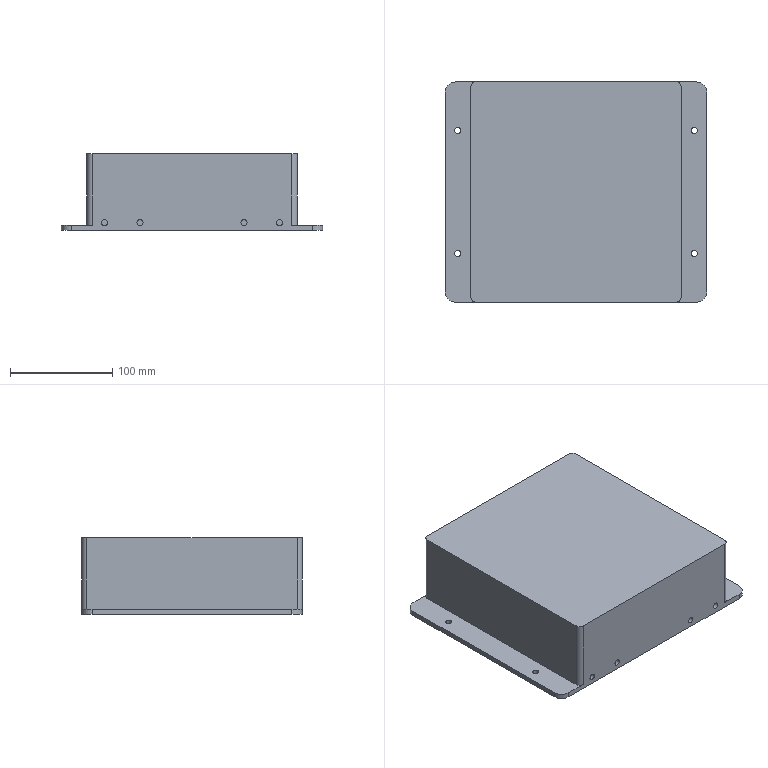NC program | NX | posted with a generic post | part box 255 x 215 x 75 mm
Lines 12222 to 12583 of 12583:
(ZLEVEL_PROFILE_COPY_1_COPY , TOOL : D10JING)
N24430 T14 M6
N24432 G54
N24434 G17 G0 G90 X-1.732 Y114.5 B0. C0. S9500 M3
N24436 G43 Z30. H14
N24438 Z-12.
N24440 G94 G1 Z-15. F1000.
N24442 X-0.866 Y113.
N24444 G3 X0. Y112.5 R1.
N24446 G1 X117.5 F1200.
N24448 G2 X132.5 Y97.5 R15.
N24450 G1 Y-97.5
N24452 G2 X117.5 Y-112.5 R15.
N24454 G1 X-117.5
N24456 G2 X-132.5 Y-97.5 R15.
N24458 G1 Y97.5
N24460 G2 X-117.5 Y112.5 R15.
N24462 G1 X0.
N24464 G3 X0.866 Y113. R1.
N24466 G1 X1.732 Y114.5
N24468 Z-14.
N24470 G0 Z30.
N24472 X-1.732
N24474 Z-27.
N24476 G1 Z-30. F1000.
N24478 X-0.866 Y113.
N24480 G3 X0. Y112.5 R1.
N24482 G1 X117.5 F1200.
N24484 G2 X132.5 Y97.5 R15.
N24486 G1 Y-97.5
N24488 G2 X117.5 Y-112.5 R15.
N24490 G1 X-117.5
N24492 G2 X-132.5 Y-97.5 R15.
N24494 G1 Y97.5
N24496 G2 X-117.5 Y112.5 R15.
N24498 G1 X0.
N24500 G3 X0.866 Y113. R1.
N24502 G1 X1.732 Y114.5
N24504 Z-29.
N24506 G0 Z30.
N24508 X-1.732
N24510 Z-42.
N24512 G1 Z-45. F1000.
N24514 X-0.866 Y113.
N24516 G3 X0. Y112.5 R1.
N24518 G1 X117.5 F1200.
N24520 G2 X132.5 Y97.5 R15.
N24522 G1 Y-97.5
N24524 G2 X117.5 Y-112.5 R15.
N24526 G1 X-117.5
N24528 G2 X-132.5 Y-97.5 R15.
N24530 G1 Y97.5
N24532 G2 X-117.5 Y112.5 R15.
N24534 G1 X0.
N24536 G3 X0.866 Y113. R1.
N24538 G1 X1.732 Y114.5
N24540 Z-44.
N24542 G0 Z30.
N24544 X-1.732
N24546 Z-57.
N24548 G1 Z-60. F1000.
N24550 X-0.866 Y113.
N24552 G3 X0. Y112.5 R1.
N24554 G1 X117.5 F1200.
N24556 G2 X132.5 Y97.5 R15.
N24558 G1 Y-97.5
N24560 G2 X117.5 Y-112.5 R15.
N24562 G1 X-117.5
N24564 G2 X-132.5 Y-97.5 R15.
N24566 G1 Y97.5
N24568 G2 X-117.5 Y112.5 R15.
N24570 G1 X0.
N24572 G3 X0.866 Y113. R1.
N24574 G1 X1.732 Y114.5
N24576 Z-59.
N24578 G0 Z30.
N24580 X-1.732
N24582 Z-72.
N24584 G1 Z-75. F1000.
N24586 X-0.866 Y113.
N24588 G3 X0. Y112.5 R1.
N24590 G1 X117.5 F1200.
N24592 G2 X132.5 Y97.5 R15.
N24594 G1 Y-97.5
N24596 G2 X117.5 Y-112.5 R15.
N24598 G1 X-117.5
N24600 G2 X-132.5 Y-97.5 R15.
N24602 G1 Y97.5
N24604 G2 X-117.5 Y112.5 R15.
N24606 G1 X0.
N24608 G3 X0.866 Y113. R1.
N24610 G1 X1.732 Y114.5
N24612 Z-74.
N24614 G0 Z30.
(ZLEVEL_PROFILE_COPY_1_COPY_COPY , TOOL : D10JING)
N24616 X95.656
N24618 Z-10.98
N24620 G1 Z-13.98 F1000.
N24622 X96.496 Y113.009
N24624 G3 X97.357 Y112.5 R1.
N24626 G1 X97.797 Y112.495 F1200.
N24628 X97.854 Y112.494
N24630 G2 X107.5 Y102.5 R10.
N24632 G1 Y-102.5
N24634 G2 X97.86 Y-112.494 R10.
N24636 G1 X97.797 Y-112.495
N24638 X97.357 Y-112.5
N24640 G3 X96.496 Y-113.009 R1.
N24642 G1 X95.656 Y-114.5
N24644 Z-12.98
N24646 G0 Z30.
N24648 X95.654 Y114.5
N24650 Z-24.96
N24652 G1 Z-27.96 F1000.
N24654 X96.496 Y113.009
N24656 G3 X97.357 Y112.5 R1.
N24658 G1 X97.797 Y112.496 F1200.
N24660 X97.854 Y112.494
N24662 G2 X107.5 Y102.5 R10.
N24664 G1 Y-102.5
N24666 G2 X97.86 Y-112.494 R10.
N24668 G1 X97.797 Y-112.496
N24670 X97.357 Y-112.5
N24672 G3 X96.496 Y-113.009 R1.
N24674 G1 X95.654 Y-114.5
N24676 Z-26.96
N24678 G0 Z30.
N24680 X95.653 Y114.5
N24682 Z-38.94
N24684 G1 Z-41.94 F1000.
N24686 X96.495 Y113.008
N24688 G3 X97.357 Y112.5 R1.
N24690 G1 X97.797 Y112.496 F1200.
N24692 X97.854 Y112.494
N24694 G2 X107.5 Y102.5 R10.
N24696 G1 Y-102.5
N24698 G2 X97.797 Y-112.496 R10.
N24700 G1 X97.357 Y-112.5
N24702 G3 X96.495 Y-113.008 R1.
N24704 G1 X95.653 Y-114.5
N24706 Z-40.94
N24708 G0 Z30.
N24710 X95.651 Y114.5
N24712 Z-52.92
N24714 G1 Z-55.92 F1000.
N24716 X96.495 Y113.008
N24718 G3 X97.357 Y112.5 R1.
N24720 G1 X97.797 Y112.496 F1200.
N24722 X97.83 Y112.495
N24724 G2 X107.5 Y102.5 R10.
N24726 G1 Y-102.5
N24728 G2 X97.797 Y-112.496 R10.001
N24730 G1 X97.357 Y-112.5
N24732 G3 X96.495 Y-113.008 R1.
N24734 G1 X95.651 Y-114.5
N24736 Z-54.92
N24738 G0 Z30.
N24740 X95.649 Y114.5
N24742 Z-66.9
N24744 G1 Z-69.9 F1000.
N24746 X96.495 Y113.007
N24748 G3 X97.357 Y112.5 R1.
N24750 G1 X97.797 Y112.496 F1200.
N24752 X97.83 Y112.495
N24754 G2 X107.5 Y102.5 R10.
N24756 G1 Y-102.5
N24758 G2 X97.797 Y-112.496 R10.001
N24760 G1 X97.357 Y-112.5
N24762 G3 X96.495 Y-113.007 R1.
N24764 G1 X95.649 Y-114.5
N24766 Z-68.9
N24768 G0 Z30.
N24770 X-95.656
N24772 Z-10.98
N24774 G1 Z-13.98 F1000.
N24776 X-96.496 Y-113.009
N24778 G3 X-97.357 Y-112.5 R1.
N24780 G1 X-97.797 Y-112.495 F1200.
N24782 X-97.854 Y-112.494
N24784 G2 X-107.5 Y-102.5 R10.
N24786 G1 Y102.5
N24788 G2 X-97.86 Y112.494 R10.
N24790 G1 X-97.818 Y112.495
N24792 X-97.357 Y112.5
N24794 G3 X-96.497 Y113.01 R1.
N24796 G1 X-95.659 Y114.5
N24798 Z-12.98
N24800 G0 Z30.
N24802 X-95.654 Y-114.5
N24804 Z-24.96
N24806 G1 Z-27.96 F1000.
N24808 X-96.496 Y-113.009
N24810 G3 X-97.357 Y-112.5 R1.
N24812 G1 X-97.797 Y-112.496 F1200.
N24814 X-97.854 Y-112.494
N24816 G2 X-107.5 Y-102.5 R10.
N24818 G1 Y102.5
N24820 G2 X-97.86 Y112.494 R10.
N24822 G1 X-97.819 Y112.495
N24824 X-97.357 Y112.5
N24826 G3 X-96.496 Y113.01 R1.
N24828 G1 X-95.658 Y114.5
N24830 Z-26.96
N24832 G0 Z30.
N24834 X-95.653 Y-114.5
N24836 Z-38.94
N24838 G1 Z-41.94 F1000.
N24840 X-96.495 Y-113.008
N24842 G3 X-97.357 Y-112.5 R1.
N24844 G1 X-97.797 Y-112.496 F1200.
N24846 X-97.854 Y-112.494
N24848 G2 X-107.5 Y-102.5 R10.
N24850 G1 Y102.5
N24852 G2 X-97.797 Y112.496 R10.
N24854 G1 X-97.357 Y112.5
N24856 G3 X-96.495 Y113.008 R1.
N24858 G1 X-95.653 Y114.5
N24860 Z-40.94
N24862 G0 Z30.
N24864 X-95.651 Y-114.5
N24866 Z-52.92
N24868 G1 Z-55.92 F1000.
N24870 X-96.495 Y-113.008
N24872 G3 X-97.357 Y-112.5 R1.
N24874 G1 X-97.797 Y-112.496 F1200.
N24876 X-97.829 Y-112.495
N24878 G2 X-107.5 Y-102.5 R10.
N24880 G1 Y102.5
N24882 G2 X-97.797 Y112.496 R10.001
N24884 G1 X-97.357 Y112.5
N24886 G3 X-96.495 Y113.008 R1.
N24888 G1 X-95.651 Y114.5
N24890 Z-54.92
N24892 G0 Z30.
N24894 X-95.649 Y-114.5
N24896 Z-66.9
N24898 G1 Z-69.9 F1000.
N24900 X-96.495 Y-113.007
N24902 G3 X-97.357 Y-112.5 R1.
N24904 G1 X-97.797 Y-112.496 F1200.
N24906 X-97.83 Y-112.495
N24908 G2 X-107.5 Y-102.5 R10.
N24910 G1 Y102.5
N24912 G2 X-97.797 Y112.496 R10.001
N24914 G1 X-97.357 Y112.5
N24916 G3 X-96.495 Y113.007 R1.
N24918 G1 X-95.649 Y114.5
N24920 Z-68.9
N24922 G0 Z30.
(FLOOR_WALL_1_COPY , TOOL : D10JING)
N24924 X-134.414 Y-99.211
N24926 Z-69.
N24928 G1 Z-70. F1000.
N24930 X-133. Y-98.395
N24932 G3 X-132.5 Y-97.529 R1.
N24934 G1 Y97.529 F1200.
N24936 G2 X-128.205 Y108.007 R15.
N24938 G1 Y-108.007
N24940 G3 X-123.911 Y-111.061 R15.
N24942 G1 Y111.061
N24944 G2 X-119.617 Y112.35 R15.
N24946 G1 Y-112.35
N24948 G3 X-117.5 Y-112.5 R15.
N24950 G1 X-115.322
N24952 Y112.5
N24954 X-111.028
N24956 Y-112.5
N24958 X-106.733
N24960 Y-107.5
N24962 G3 X-102.439 Y-111.766 R10.5
N24964 G1 Y-112.5
N24966 G2 X-102.939 Y-113.366 R1.
N24968 G1 X-104.903 Y-114.5
N24970 Z-69.
N24972 G0 X-106.733 Y-107.5
N24974 G1 Z-70. F1000.
N24976 G2 X-108. Y-102.5 R10.5
N24978 G1 Y102.5
N24980 G2 X-106.733 Y107.5 R10.5
N24982 G1 Y112.5 F1200.
N24984 X-102.439
N24986 Y111.766
N24988 Z-69.
N24990 G0 Z30.
N24992 X-96.34 Y-114.5
N24994 Z-69.
N24996 G1 Z-70. F1000.
N24998 X-97.104 Y-113.028
N25000 G3 X-97.947 Y-112.49 R1.
N25002 G2 X-107.5 Y-102.5 R10. F1200.
N25004 G1 Y102.5
N25006 G2 X-97.947 Y112.49 R10.
N25008 G3 X-97.104 Y113.028 R1.
N25010 G1 X-96.34 Y114.5
N25012 Z-69.
N25014 G0 Z30.
N25016 X104.269 Y-114.5
N25018 Z-69.
N25020 G1 Z-70. F1000.
N25022 X106.233 Y-113.366
N25024 G3 X106.733 Y-112.5 R1.
N25026 G1 Y-107.5 F1200.
N25028 G3 X108. Y-102.5 R10.5
N25030 G1 Y102.5
N25032 G3 X106.733 Y107.5 R10.5
N25034 G1 Y112.5
N25036 X110.925
N25038 Y-112.5
N25040 X115.117
N25042 Y112.5
N25044 X117.5
N25046 G2 X119.308 Y112.391 R15.
N25048 G1 Y-112.391
N25050 G3 X123.5 Y-111.248 R15.
N25052 G1 Y111.248
N25054 G3 X123. Y112.114 R1.
N25056 G1 X123.488 Y113.41
N25058 Z-69.
N25060 G0 X96.34 Y114.5
N25062 G1 Z-70. F1000.
N25064 X97.104 Y113.028
N25066 G3 X97.947 Y112.49 R1.
N25068 G2 X107.5 Y102.5 R10. F1200.
N25070 G1 Y-102.5
N25072 G2 X97.947 Y-112.49 R10.
N25074 G3 X97.104 Y-113.028 R1.
N25076 G1 X96.34 Y-114.5
N25078 Z-69.
N25080 G0 Z30.
N25082 M5
(PLANAR_MILL_COPY_COPY_COPY_COPY , TOOL : D6A45)
N25084 T01 M6
N25086 G54
N25088 G17 G0 G90 X-105.1 Y-1.27 B0. C0. S9500 M3
N25090 G43 Z30. H1
N25092 Z0.
N25094 G94 G1 Z-1.5 F1250.
N25096 X-104.4 Y-0.866
N25098 G3 X-103.9 Y0. R1.
N25100 G1 Y102.5
N25102 G2 X-97.5 Y108.9 R6.4
N25104 G1 X97.5
N25106 G2 X103.9 Y102.5 R6.4
N25108 G1 Y-102.5
N25110 G2 X97.5 Y-108.9 R6.4
N25112 G1 X-97.5
N25114 G2 X-103.9 Y-102.5 R6.4
N25116 G1 Y0.
N25118 G3 X-104.4 Y0.866 R1.
N25120 G1 X-105.1 Y1.27
N25122 Z0.
N25124 G0 Z30.
N25126 M5
N25128 M2